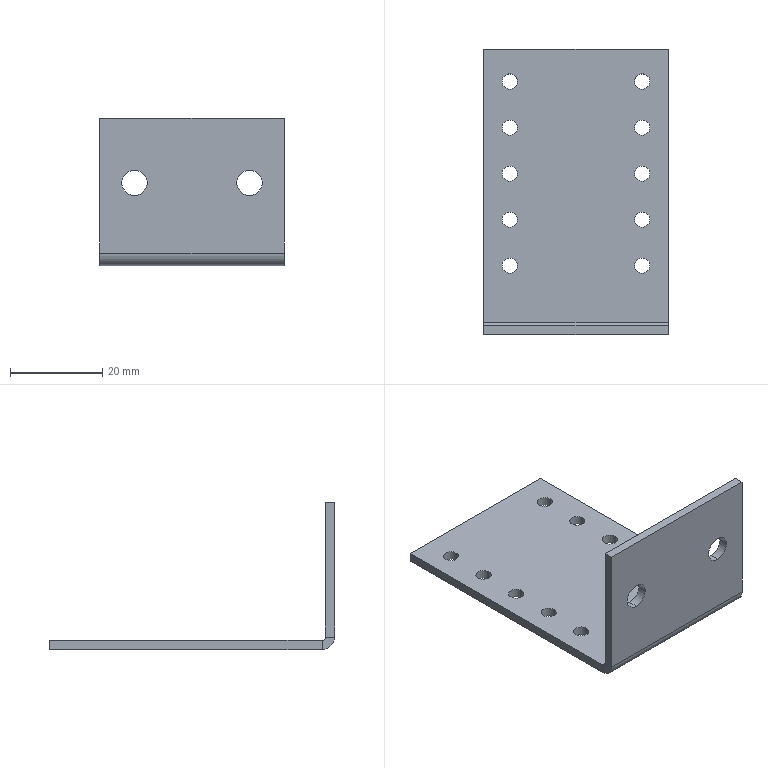Part | STEP file | 1 solid | 38 faces | box 40 x 62 x 32 mm | volume 7034 mm3 | cylinder 26 | plane 12 | commonest cylinder face diameters 3.3 x20 5.5 x4 1.473 x1 5.473 x1